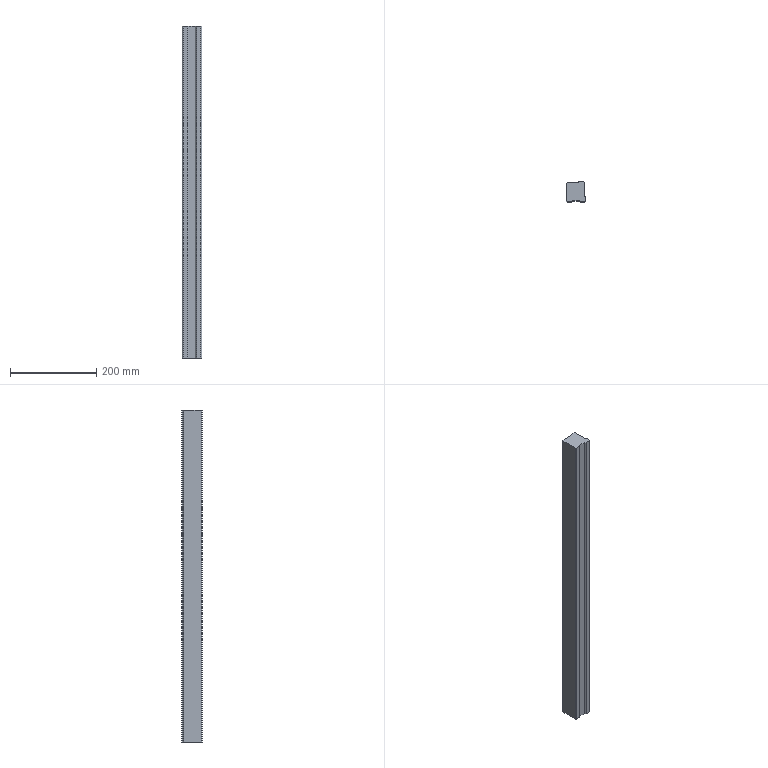Part | STEP file | Platform guide seat (default) | 1 solid | 18 faces | box 45 x 47 x 770 mm | volume 1483790 mm3 | plane 18
STEP:
#1=CARTESIAN_POINT('',(10.5,-23.5,-385.));
#2=VERTEX_POINT('',#1);
#3=CARTESIAN_POINT('',(20.5,-23.5,-385.));
#4=VERTEX_POINT('',#3);
#5=CARTESIAN_POINT('',(-22.5,-23.5,-385.));
#6=DIRECTION('',(1.,0.,0.));
#7=VECTOR('',#6,1000.);
#8=LINE('',#5,#7);
#9=EDGE_CURVE('',#2,#4,#8,.T.);
#10=ORIENTED_EDGE('',*,*,#9,.T.);
#11=CARTESIAN_POINT('',(20.5,-23.5,385.));
#12=VERTEX_POINT('',#11);
#13=CARTESIAN_POINT('',(20.5,-23.5,385.));
#14=DIRECTION('',(0.,0.,1.));
#15=VECTOR('',#14,1000.);
#16=LINE('',#13,#15);
#17=EDGE_CURVE('',#4,#12,#16,.T.);
#18=ORIENTED_EDGE('',*,*,#17,.T.);
#19=CARTESIAN_POINT('',(10.5,-23.5,385.));
#20=VERTEX_POINT('',#19);
#21=CARTESIAN_POINT('',(-22.5,-23.5,385.));
#22=DIRECTION('',(1.,0.,0.));
#23=VECTOR('',#22,1000.);
#24=LINE('',#21,#23);
#25=EDGE_CURVE('',#20,#12,#24,.T.);
#26=ORIENTED_EDGE('',*,*,#25,.F.);
#27=CARTESIAN_POINT('',(10.5,-23.5,-385.));
#28=DIRECTION('',(0.,0.,1.));
#29=VECTOR('',#28,1000.);
#30=LINE('',#27,#29);
#31=EDGE_CURVE('',#2,#20,#30,.T.);
#32=ORIENTED_EDGE('',*,*,#31,.F.);
#33=EDGE_LOOP('',(#10,#18,#26,#32));
#34=FACE_OUTER_BOUND('',#33,.T.);
#35=CARTESIAN_POINT('',(-22.5,-23.5,385.));
#36=DIRECTION('',(0.,1.,0.));
#37=DIRECTION('',(0.,0.,1.));
#38=AXIS2_PLACEMENT_3D('',#35,#36,#37);
#39=PLANE('',#38);
#40=ADVANCED_FACE('',(#34),#39,.F.);
#41=CARTESIAN_POINT('',(22.5,-21.5,385.));
#42=VERTEX_POINT('',#41);
#43=CARTESIAN_POINT('',(22.5,-11.5,385.));
#44=VERTEX_POINT('',#43);
#45=CARTESIAN_POINT('',(22.5,23.5,385.));
#46=DIRECTION('',(0.,1.,0.));
#47=VECTOR('',#46,1000.);
#48=LINE('',#45,#47);
#49=EDGE_CURVE('',#42,#44,#48,.T.);
#50=ORIENTED_EDGE('',*,*,#49,.F.);
#51=CARTESIAN_POINT('',(22.5,-21.5,-385.));
#52=VERTEX_POINT('',#51);
#53=CARTESIAN_POINT('',(22.5,-21.5,385.));
#54=DIRECTION('',(0.,0.,-1.));
#55=VECTOR('',#54,1000.);
#56=LINE('',#53,#55);
#57=EDGE_CURVE('',#42,#52,#56,.T.);
#58=ORIENTED_EDGE('',*,*,#57,.T.);
#59=CARTESIAN_POINT('',(22.5,-11.5,-385.));
#60=VERTEX_POINT('',#59);
#61=CARTESIAN_POINT('',(22.5,23.5,-385.));
#62=DIRECTION('',(0.,1.,0.));
#63=VECTOR('',#62,1000.);
#64=LINE('',#61,#63);
#65=EDGE_CURVE('',#52,#60,#64,.T.);
#66=ORIENTED_EDGE('',*,*,#65,.T.);
#67=CARTESIAN_POINT('',(22.5,-11.5,-385.));
#68=DIRECTION('',(0.,0.,1.));
#69=VECTOR('',#68,1000.);
#70=LINE('',#67,#69);
#71=EDGE_CURVE('',#60,#44,#70,.T.);
#72=ORIENTED_EDGE('',*,*,#71,.T.);
#73=EDGE_LOOP('',(#50,#58,#66,#72));
#74=FACE_OUTER_BOUND('',#73,.T.);
#75=CARTESIAN_POINT('',(22.5,23.5,385.));
#76=DIRECTION('',(-1.,0.,0.));
#77=DIRECTION('',(0.,-1.,0.));
#78=AXIS2_PLACEMENT_3D('',#75,#76,#77);
#79=PLANE('',#78);
#80=ADVANCED_FACE('',(#74),#79,.F.);
#81=CARTESIAN_POINT('',(18.5,23.5,385.));
#82=VERTEX_POINT('',#81);
#83=CARTESIAN_POINT('',(5.5,23.5,385.));
#84=VERTEX_POINT('',#83);
#85=CARTESIAN_POINT('',(-22.5,23.5,385.));
#86=DIRECTION('',(-1.,0.,0.));
#87=VECTOR('',#86,1000.);
#88=LINE('',#85,#87);
#89=EDGE_CURVE('',#82,#84,#88,.T.);
#90=ORIENTED_EDGE('',*,*,#89,.F.);
#91=CARTESIAN_POINT('',(18.5,23.5,-385.));
#92=VERTEX_POINT('',#91);
#93=CARTESIAN_POINT('',(18.5,23.5,385.));
#94=DIRECTION('',(0.,0.,-1.));
#95=VECTOR('',#94,1000.);
#96=LINE('',#93,#95);
#97=EDGE_CURVE('',#82,#92,#96,.T.);
#98=ORIENTED_EDGE('',*,*,#97,.T.);
#99=CARTESIAN_POINT('',(5.5,23.5,-385.));
#100=VERTEX_POINT('',#99);
#101=CARTESIAN_POINT('',(-22.5,23.5,-385.));
#102=DIRECTION('',(-1.,0.,0.));
#103=VECTOR('',#102,1000.);
#104=LINE('',#101,#103);
#105=EDGE_CURVE('',#92,#100,#104,.T.);
#106=ORIENTED_EDGE('',*,*,#105,.T.);
#107=CARTESIAN_POINT('',(5.5,23.5,-385.));
#108=DIRECTION('',(0.,0.,1.));
#109=VECTOR('',#108,1000.);
#110=LINE('',#107,#109);
#111=EDGE_CURVE('',#100,#84,#110,.T.);
#112=ORIENTED_EDGE('',*,*,#111,.T.);
#113=EDGE_LOOP('',(#90,#98,#106,#112));
#114=FACE_OUTER_BOUND('',#113,.T.);
#115=CARTESIAN_POINT('',(-22.5,23.5,385.));
#116=DIRECTION('',(0.,-1.,0.));
#117=DIRECTION('',(0.,0.,-1.));
#118=AXIS2_PLACEMENT_3D('',#115,#116,#117);
#119=PLANE('',#118);
#120=ADVANCED_FACE('',(#114),#119,.F.);
#121=CARTESIAN_POINT('',(-22.5,19.5,385.));
#122=VERTEX_POINT('',#121);
#123=CARTESIAN_POINT('',(-22.5,-21.5,385.));
#124=VERTEX_POINT('',#123);
#125=CARTESIAN_POINT('',(-22.5,23.5,385.));
#126=DIRECTION('',(0.,-1.,0.));
#127=VECTOR('',#126,1000.);
#128=LINE('',#125,#127);
#129=EDGE_CURVE('',#122,#124,#128,.T.);
#130=ORIENTED_EDGE('',*,*,#129,.F.);
#131=CARTESIAN_POINT('',(-22.5,19.5,-385.));
#132=VERTEX_POINT('',#131);
#133=CARTESIAN_POINT('',(-22.5,19.5,385.));
#134=DIRECTION('',(0.,0.,-1.));
#135=VECTOR('',#134,1000.);
#136=LINE('',#133,#135);
#137=EDGE_CURVE('',#122,#132,#136,.T.);
#138=ORIENTED_EDGE('',*,*,#137,.T.);
#139=CARTESIAN_POINT('',(-22.5,-21.5,-385.));
#140=VERTEX_POINT('',#139);
#141=CARTESIAN_POINT('',(-22.5,23.5,-385.));
#142=DIRECTION('',(0.,-1.,0.));
#143=VECTOR('',#142,1000.);
#144=LINE('',#141,#143);
#145=EDGE_CURVE('',#132,#140,#144,.T.);
#146=ORIENTED_EDGE('',*,*,#145,.T.);
#147=CARTESIAN_POINT('',(-22.5,-21.5,385.));
#148=DIRECTION('',(0.,0.,1.));
#149=VECTOR('',#148,1000.);
#150=LINE('',#147,#149);
#151=EDGE_CURVE('',#140,#124,#150,.T.);
#152=ORIENTED_EDGE('',*,*,#151,.T.);
#153=EDGE_LOOP('',(#130,#138,#146,#152));
#154=FACE_OUTER_BOUND('',#153,.T.);
#155=CARTESIAN_POINT('',(-22.5,23.5,385.));
#156=DIRECTION('',(1.,0.,0.));
#157=DIRECTION('',(0.,1.,0.));
#158=AXIS2_PLACEMENT_3D('',#155,#156,#157);
#159=PLANE('',#158);
#160=ADVANCED_FACE('',(#154),#159,.F.);
#161=CARTESIAN_POINT('',(-20.5,-23.5,385.));
#162=VERTEX_POINT('',#161);
#163=CARTESIAN_POINT('',(-10.5,-23.5,385.));
#164=VERTEX_POINT('',#163);
#165=CARTESIAN_POINT('',(-22.5,-23.5,385.));
#166=DIRECTION('',(1.,0.,0.));
#167=VECTOR('',#166,1000.);
#168=LINE('',#165,#167);
#169=EDGE_CURVE('',#162,#164,#168,.T.);
#170=ORIENTED_EDGE('',*,*,#169,.F.);
#171=CARTESIAN_POINT('',(-20.5,-23.5,-385.));
#172=VERTEX_POINT('',#171);
#173=CARTESIAN_POINT('',(-20.5,-23.5,385.));
#174=DIRECTION('',(0.,0.,-1.));
#175=VECTOR('',#174,1000.);
#176=LINE('',#173,#175);
#177=EDGE_CURVE('',#162,#172,#176,.T.);
#178=ORIENTED_EDGE('',*,*,#177,.T.);
#179=CARTESIAN_POINT('',(-10.5,-23.5,-385.));
#180=VERTEX_POINT('',#179);
#181=CARTESIAN_POINT('',(-22.5,-23.5,-385.));
#182=DIRECTION('',(1.,0.,0.));
#183=VECTOR('',#182,1000.);
#184=LINE('',#181,#183);
#185=EDGE_CURVE('',#172,#180,#184,.T.);
#186=ORIENTED_EDGE('',*,*,#185,.T.);
#187=CARTESIAN_POINT('',(-10.5,-23.5,-385.));
#188=DIRECTION('',(0.,0.,1.));
#189=VECTOR('',#188,1000.);
#190=LINE('',#187,#189);
#191=EDGE_CURVE('',#180,#164,#190,.T.);
#192=ORIENTED_EDGE('',*,*,#191,.T.);
#193=EDGE_LOOP('',(#170,#178,#186,#192));
#194=FACE_OUTER_BOUND('',#193,.T.);
#195=CARTESIAN_POINT('',(-22.5,-23.5,385.));
#196=DIRECTION('',(0.,1.,0.));
#197=DIRECTION('',(0.,0.,1.));
#198=AXIS2_PLACEMENT_3D('',#195,#196,#197);
#199=PLANE('',#198);
#200=ADVANCED_FACE('',(#194),#199,.F.);
#201=CARTESIAN_POINT('',(20.5,21.5,385.));
#202=VERTEX_POINT('',#201);
#203=CARTESIAN_POINT('',(20.5,-11.5,385.));
#204=VERTEX_POINT('',#203);
#205=CARTESIAN_POINT('',(20.5,23.5,385.));
#206=DIRECTION('',(0.,-1.,0.));
#207=VECTOR('',#206,1000.);
#208=LINE('',#205,#207);
#209=EDGE_CURVE('',#202,#204,#208,.T.);
#210=ORIENTED_EDGE('',*,*,#209,.F.);
#211=CARTESIAN_POINT('',(21.,21.,385.));
#212=DIRECTION('',(-0.7071,0.7071,0.));
#213=VECTOR('',#212,1000.);
#214=LINE('',#211,#213);
#215=EDGE_CURVE('',#202,#82,#214,.T.);
#216=ORIENTED_EDGE('',*,*,#215,.T.);
#217=ORIENTED_EDGE('',*,*,#89,.T.);
#218=CARTESIAN_POINT('',(5.5,21.5,385.));
#219=VERTEX_POINT('',#218);
#220=CARTESIAN_POINT('',(5.5,23.5,385.));
#221=DIRECTION('',(0.,1.,0.));
#222=VECTOR('',#221,1000.);
#223=LINE('',#220,#222);
#224=EDGE_CURVE('',#219,#84,#223,.T.);
#225=ORIENTED_EDGE('',*,*,#224,.F.);
#226=CARTESIAN_POINT('',(-20.5,21.5,385.));
#227=VERTEX_POINT('',#226);
#228=CARTESIAN_POINT('',(-22.5,21.5,385.));
#229=DIRECTION('',(1.,0.,0.));
#230=VECTOR('',#229,1000.);
#231=LINE('',#228,#230);
#232=EDGE_CURVE('',#227,#219,#231,.T.);
#233=ORIENTED_EDGE('',*,*,#232,.F.);
#234=CARTESIAN_POINT('',(-21.,21.,385.));
#235=DIRECTION('',(-0.7071,-0.7071,0.));
#236=VECTOR('',#235,1000.);
#237=LINE('',#234,#236);
#238=EDGE_CURVE('',#227,#122,#237,.T.);
#239=ORIENTED_EDGE('',*,*,#238,.T.);
#240=ORIENTED_EDGE('',*,*,#129,.T.);
#241=CARTESIAN_POINT('',(-22.,-22.,385.));
#242=DIRECTION('',(0.7071,-0.7071,0.));
#243=VECTOR('',#242,1000.);
#244=LINE('',#241,#243);
#245=EDGE_CURVE('',#124,#162,#244,.T.);
#246=ORIENTED_EDGE('',*,*,#245,.T.);
#247=ORIENTED_EDGE('',*,*,#169,.T.);
#248=CARTESIAN_POINT('',(-7.5,-20.5,385.));
#249=VERTEX_POINT('',#248);
#250=CARTESIAN_POINT('',(-7.5,-20.5,385.));
#251=DIRECTION('',(-0.7071,-0.7071,0.));
#252=VECTOR('',#251,1000.);
#253=LINE('',#250,#252);
#254=EDGE_CURVE('',#249,#164,#253,.T.);
#255=ORIENTED_EDGE('',*,*,#254,.F.);
#256=CARTESIAN_POINT('',(7.5,-20.5,385.));
#257=VERTEX_POINT('',#256);
#258=CARTESIAN_POINT('',(-7.5,-20.5,385.));
#259=DIRECTION('',(-1.,0.,0.));
#260=VECTOR('',#259,1000.);
#261=LINE('',#258,#260);
#262=EDGE_CURVE('',#257,#249,#261,.T.);
#263=ORIENTED_EDGE('',*,*,#262,.F.);
#264=CARTESIAN_POINT('',(7.5,-20.5,385.));
#265=DIRECTION('',(-0.7071,0.7071,0.));
#266=VECTOR('',#265,1000.);
#267=LINE('',#264,#266);
#268=EDGE_CURVE('',#20,#257,#267,.T.);
#269=ORIENTED_EDGE('',*,*,#268,.F.);
#270=ORIENTED_EDGE('',*,*,#25,.T.);
#271=CARTESIAN_POINT('',(22.,-22.,385.));
#272=DIRECTION('',(0.7071,0.7071,0.));
#273=VECTOR('',#272,1000.);
#274=LINE('',#271,#273);
#275=EDGE_CURVE('',#12,#42,#274,.T.);
#276=ORIENTED_EDGE('',*,*,#275,.T.);
#277=ORIENTED_EDGE('',*,*,#49,.T.);
#278=CARTESIAN_POINT('',(22.5,-11.5,385.));
#279=DIRECTION('',(1.,0.,0.));
#280=VECTOR('',#279,1000.);
#281=LINE('',#278,#280);
#282=EDGE_CURVE('',#204,#44,#281,.T.);
#283=ORIENTED_EDGE('',*,*,#282,.F.);
#284=EDGE_LOOP('',(#210,#216,#217,#225,#233,#239,#240,#246,#247,#255,#263,#269,#270,#276,#277,#283));
#285=FACE_OUTER_BOUND('',#284,.T.);
#286=CARTESIAN_POINT('',(0.,0.,385.));
#287=DIRECTION('',(0.,0.,1.));
#288=DIRECTION('',(1.,0.,0.));
#289=AXIS2_PLACEMENT_3D('',#286,#287,#288);
#290=PLANE('',#289);
#291=ADVANCED_FACE('',(#285),#290,.T.);
#292=ORIENTED_EDGE('',*,*,#105,.F.);
#293=CARTESIAN_POINT('',(20.5,21.5,-385.));
#294=VERTEX_POINT('',#293);
#295=CARTESIAN_POINT('',(20.5,21.5,-385.));
#296=DIRECTION('',(0.7071,-0.7071,0.));
#297=VECTOR('',#296,1000.);
#298=LINE('',#295,#297);
#299=EDGE_CURVE('',#92,#294,#298,.T.);
#300=ORIENTED_EDGE('',*,*,#299,.T.);
#301=CARTESIAN_POINT('',(20.5,-11.5,-385.));
#302=VERTEX_POINT('',#301);
#303=CARTESIAN_POINT('',(20.5,23.5,-385.));
#304=DIRECTION('',(0.,-1.,0.));
#305=VECTOR('',#304,1000.);
#306=LINE('',#303,#305);
#307=EDGE_CURVE('',#294,#302,#306,.T.);
#308=ORIENTED_EDGE('',*,*,#307,.T.);
#309=CARTESIAN_POINT('',(22.5,-11.5,-385.));
#310=DIRECTION('',(1.,0.,0.));
#311=VECTOR('',#310,1000.);
#312=LINE('',#309,#311);
#313=EDGE_CURVE('',#302,#60,#312,.T.);
#314=ORIENTED_EDGE('',*,*,#313,.T.);
#315=ORIENTED_EDGE('',*,*,#65,.F.);
#316=CARTESIAN_POINT('',(22.5,-21.5,-385.));
#317=DIRECTION('',(-0.7071,-0.7071,0.));
#318=VECTOR('',#317,1000.);
#319=LINE('',#316,#318);
#320=EDGE_CURVE('',#52,#4,#319,.T.);
#321=ORIENTED_EDGE('',*,*,#320,.T.);
#322=ORIENTED_EDGE('',*,*,#9,.F.);
#323=CARTESIAN_POINT('',(7.5,-20.5,-385.));
#324=VERTEX_POINT('',#323);
#325=CARTESIAN_POINT('',(7.5,-20.5,-385.));
#326=DIRECTION('',(-0.7071,0.7071,0.));
#327=VECTOR('',#326,1000.);
#328=LINE('',#325,#327);
#329=EDGE_CURVE('',#2,#324,#328,.T.);
#330=ORIENTED_EDGE('',*,*,#329,.T.);
#331=CARTESIAN_POINT('',(-7.5,-20.5,-385.));
#332=VERTEX_POINT('',#331);
#333=CARTESIAN_POINT('',(-7.5,-20.5,-385.));
#334=DIRECTION('',(-1.,0.,0.));
#335=VECTOR('',#334,1000.);
#336=LINE('',#333,#335);
#337=EDGE_CURVE('',#324,#332,#336,.T.);
#338=ORIENTED_EDGE('',*,*,#337,.T.);
#339=CARTESIAN_POINT('',(-7.5,-20.5,-385.));
#340=DIRECTION('',(-0.7071,-0.7071,0.));
#341=VECTOR('',#340,1000.);
#342=LINE('',#339,#341);
#343=EDGE_CURVE('',#332,#180,#342,.T.);
#344=ORIENTED_EDGE('',*,*,#343,.T.);
#345=ORIENTED_EDGE('',*,*,#185,.F.);
#346=CARTESIAN_POINT('',(-20.5,-23.5,-385.));
#347=DIRECTION('',(-0.7071,0.7071,0.));
#348=VECTOR('',#347,1000.);
#349=LINE('',#346,#348);
#350=EDGE_CURVE('',#172,#140,#349,.T.);
#351=ORIENTED_EDGE('',*,*,#350,.T.);
#352=ORIENTED_EDGE('',*,*,#145,.F.);
#353=CARTESIAN_POINT('',(-20.5,21.5,-385.));
#354=VERTEX_POINT('',#353);
#355=CARTESIAN_POINT('',(-20.5,21.5,-385.));
#356=DIRECTION('',(0.7071,0.7071,0.));
#357=VECTOR('',#356,1000.);
#358=LINE('',#355,#357);
#359=EDGE_CURVE('',#132,#354,#358,.T.);
#360=ORIENTED_EDGE('',*,*,#359,.T.);
#361=CARTESIAN_POINT('',(5.5,21.5,-385.));
#362=VERTEX_POINT('',#361);
#363=CARTESIAN_POINT('',(-22.5,21.5,-385.));
#364=DIRECTION('',(1.,0.,0.));
#365=VECTOR('',#364,1000.);
#366=LINE('',#363,#365);
#367=EDGE_CURVE('',#354,#362,#366,.T.);
#368=ORIENTED_EDGE('',*,*,#367,.T.);
#369=CARTESIAN_POINT('',(5.5,23.5,-385.));
#370=DIRECTION('',(0.,1.,0.));
#371=VECTOR('',#370,1000.);
#372=LINE('',#369,#371);
#373=EDGE_CURVE('',#362,#100,#372,.T.);
#374=ORIENTED_EDGE('',*,*,#373,.T.);
#375=EDGE_LOOP('',(#292,#300,#308,#314,#315,#321,#322,#330,#338,#344,#345,#351,#352,#360,#368,#374));
#376=FACE_OUTER_BOUND('',#375,.T.);
#377=CARTESIAN_POINT('',(0.,0.,-385.));
#378=DIRECTION('',(0.,0.,1.));
#379=DIRECTION('',(1.,0.,0.));
#380=AXIS2_PLACEMENT_3D('',#377,#378,#379);
#381=PLANE('',#380);
#382=ADVANCED_FACE('',(#376),#381,.F.);
#383=ORIENTED_EDGE('',*,*,#224,.T.);
#384=ORIENTED_EDGE('',*,*,#111,.F.);
#385=ORIENTED_EDGE('',*,*,#373,.F.);
#386=CARTESIAN_POINT('',(5.5,21.5,-385.));
#387=DIRECTION('',(0.,0.,1.));
#388=VECTOR('',#387,1000.);
#389=LINE('',#386,#388);
#390=EDGE_CURVE('',#362,#219,#389,.T.);
#391=ORIENTED_EDGE('',*,*,#390,.T.);
#392=EDGE_LOOP('',(#383,#384,#385,#391));
#393=FACE_OUTER_BOUND('',#392,.T.);
#394=CARTESIAN_POINT('',(5.5,23.5,-385.));
#395=DIRECTION('',(1.,0.,0.));
#396=DIRECTION('',(0.,0.,-1.));
#397=AXIS2_PLACEMENT_3D('',#394,#395,#396);
#398=PLANE('',#397);
#399=ADVANCED_FACE('',(#393),#398,.F.);
#400=ORIENTED_EDGE('',*,*,#367,.F.);
#401=CARTESIAN_POINT('',(-20.5,21.5,-385.));
#402=DIRECTION('',(0.,0.,1.));
#403=VECTOR('',#402,1000.);
#404=LINE('',#401,#403);
#405=EDGE_CURVE('',#354,#227,#404,.T.);
#406=ORIENTED_EDGE('',*,*,#405,.T.);
#407=ORIENTED_EDGE('',*,*,#232,.T.);
#408=ORIENTED_EDGE('',*,*,#390,.F.);
#409=EDGE_LOOP('',(#400,#406,#407,#408));
#410=FACE_OUTER_BOUND('',#409,.T.);
#411=CARTESIAN_POINT('',(-22.5,21.5,-385.));
#412=DIRECTION('',(0.,-1.,0.));
#413=DIRECTION('',(0.,0.,-1.));
#414=AXIS2_PLACEMENT_3D('',#411,#412,#413);
#415=PLANE('',#414);
#416=ADVANCED_FACE('',(#410),#415,.F.);
#417=ORIENTED_EDGE('',*,*,#282,.T.);
#418=ORIENTED_EDGE('',*,*,#71,.F.);
#419=ORIENTED_EDGE('',*,*,#313,.F.);
#420=CARTESIAN_POINT('',(20.5,-11.5,-385.));
#421=DIRECTION('',(0.,0.,1.));
#422=VECTOR('',#421,1000.);
#423=LINE('',#420,#422);
#424=EDGE_CURVE('',#302,#204,#423,.T.);
#425=ORIENTED_EDGE('',*,*,#424,.T.);
#426=EDGE_LOOP('',(#417,#418,#419,#425));
#427=FACE_OUTER_BOUND('',#426,.T.);
#428=CARTESIAN_POINT('',(22.5,-11.5,-385.));
#429=DIRECTION('',(0.,-1.,0.));
#430=DIRECTION('',(0.,0.,-1.));
#431=AXIS2_PLACEMENT_3D('',#428,#429,#430);
#432=PLANE('',#431);
#433=ADVANCED_FACE('',(#427),#432,.F.);
#434=ORIENTED_EDGE('',*,*,#307,.F.);
#435=CARTESIAN_POINT('',(20.5,21.5,-385.));
#436=DIRECTION('',(0.,0.,1.));
#437=VECTOR('',#436,1000.);
#438=LINE('',#435,#437);
#439=EDGE_CURVE('',#294,#202,#438,.T.);
#440=ORIENTED_EDGE('',*,*,#439,.T.);
#441=ORIENTED_EDGE('',*,*,#209,.T.);
#442=ORIENTED_EDGE('',*,*,#424,.F.);
#443=EDGE_LOOP('',(#434,#440,#441,#442));
#444=FACE_OUTER_BOUND('',#443,.T.);
#445=CARTESIAN_POINT('',(20.5,23.5,-385.));
#446=DIRECTION('',(-1.,0.,0.));
#447=DIRECTION('',(0.,-1.,0.));
#448=AXIS2_PLACEMENT_3D('',#445,#446,#447);
#449=PLANE('',#448);
#450=ADVANCED_FACE('',(#444),#449,.F.);
#451=ORIENTED_EDGE('',*,*,#268,.T.);
#452=CARTESIAN_POINT('',(7.5,-20.5,-385.));
#453=DIRECTION('',(0.,0.,1.));
#454=VECTOR('',#453,1000.);
#455=LINE('',#452,#454);
#456=EDGE_CURVE('',#324,#257,#455,.T.);
#457=ORIENTED_EDGE('',*,*,#456,.F.);
#458=ORIENTED_EDGE('',*,*,#329,.F.);
#459=ORIENTED_EDGE('',*,*,#31,.T.);
#460=EDGE_LOOP('',(#451,#457,#458,#459));
#461=FACE_OUTER_BOUND('',#460,.T.);
#462=CARTESIAN_POINT('',(7.5,-20.5,-385.));
#463=DIRECTION('',(0.7071,0.7071,0.));
#464=DIRECTION('',(-0.7071,0.7071,0.));
#465=AXIS2_PLACEMENT_3D('',#462,#463,#464);
#466=PLANE('',#465);
#467=ADVANCED_FACE('',(#461),#466,.F.);
#468=ORIENTED_EDGE('',*,*,#254,.T.);
#469=ORIENTED_EDGE('',*,*,#191,.F.);
#470=ORIENTED_EDGE('',*,*,#343,.F.);
#471=CARTESIAN_POINT('',(-7.5,-20.5,-385.));
#472=DIRECTION('',(0.,0.,1.));
#473=VECTOR('',#472,1000.);
#474=LINE('',#471,#473);
#475=EDGE_CURVE('',#332,#249,#474,.T.);
#476=ORIENTED_EDGE('',*,*,#475,.T.);
#477=EDGE_LOOP('',(#468,#469,#470,#476));
#478=FACE_OUTER_BOUND('',#477,.T.);
#479=CARTESIAN_POINT('',(-7.5,-20.5,-385.));
#480=DIRECTION('',(-0.7071,0.7071,0.));
#481=DIRECTION('',(-0.7071,-0.7071,0.));
#482=AXIS2_PLACEMENT_3D('',#479,#480,#481);
#483=PLANE('',#482);
#484=ADVANCED_FACE('',(#478),#483,.F.);
#485=ORIENTED_EDGE('',*,*,#262,.T.);
#486=ORIENTED_EDGE('',*,*,#475,.F.);
#487=ORIENTED_EDGE('',*,*,#337,.F.);
#488=ORIENTED_EDGE('',*,*,#456,.T.);
#489=EDGE_LOOP('',(#485,#486,#487,#488));
#490=FACE_OUTER_BOUND('',#489,.T.);
#491=CARTESIAN_POINT('',(-7.5,-20.5,-385.));
#492=DIRECTION('',(0.,1.,0.));
#493=DIRECTION('',(0.,0.,1.));
#494=AXIS2_PLACEMENT_3D('',#491,#492,#493);
#495=PLANE('',#494);
#496=ADVANCED_FACE('',(#490),#495,.F.);
#497=ORIENTED_EDGE('',*,*,#299,.F.);
#498=ORIENTED_EDGE('',*,*,#97,.F.);
#499=ORIENTED_EDGE('',*,*,#215,.F.);
#500=ORIENTED_EDGE('',*,*,#439,.F.);
#501=EDGE_LOOP('',(#497,#498,#499,#500));
#502=FACE_OUTER_BOUND('',#501,.T.);
#503=CARTESIAN_POINT('',(20.5,21.5,-385.));
#504=DIRECTION('',(-0.7071,-0.7071,0.));
#505=DIRECTION('',(0.,0.,1.));
#506=AXIS2_PLACEMENT_3D('',#503,#504,#505);
#507=PLANE('',#506);
#508=ADVANCED_FACE('',(#502),#507,.F.);
#509=ORIENTED_EDGE('',*,*,#359,.F.);
#510=ORIENTED_EDGE('',*,*,#137,.F.);
#511=ORIENTED_EDGE('',*,*,#238,.F.);
#512=ORIENTED_EDGE('',*,*,#405,.F.);
#513=EDGE_LOOP('',(#509,#510,#511,#512));
#514=FACE_OUTER_BOUND('',#513,.T.);
#515=CARTESIAN_POINT('',(-20.5,21.5,-385.));
#516=DIRECTION('',(0.7071,-0.7071,0.));
#517=DIRECTION('',(0.,0.,1.));
#518=AXIS2_PLACEMENT_3D('',#515,#516,#517);
#519=PLANE('',#518);
#520=ADVANCED_FACE('',(#514),#519,.F.);
#521=ORIENTED_EDGE('',*,*,#245,.F.);
#522=ORIENTED_EDGE('',*,*,#151,.F.);
#523=ORIENTED_EDGE('',*,*,#350,.F.);
#524=ORIENTED_EDGE('',*,*,#177,.F.);
#525=EDGE_LOOP('',(#521,#522,#523,#524));
#526=FACE_OUTER_BOUND('',#525,.T.);
#527=CARTESIAN_POINT('',(-20.5,-23.5,385.));
#528=DIRECTION('',(0.7071,0.7071,0.));
#529=DIRECTION('',(0.,0.,-1.));
#530=AXIS2_PLACEMENT_3D('',#527,#528,#529);
#531=PLANE('',#530);
#532=ADVANCED_FACE('',(#526),#531,.F.);
#533=ORIENTED_EDGE('',*,*,#275,.F.);
#534=ORIENTED_EDGE('',*,*,#17,.F.);
#535=ORIENTED_EDGE('',*,*,#320,.F.);
#536=ORIENTED_EDGE('',*,*,#57,.F.);
#537=EDGE_LOOP('',(#533,#534,#535,#536));
#538=FACE_OUTER_BOUND('',#537,.T.);
#539=CARTESIAN_POINT('',(22.5,-21.5,385.));
#540=DIRECTION('',(-0.7071,0.7071,0.));
#541=DIRECTION('',(0.,0.,-1.));
#542=AXIS2_PLACEMENT_3D('',#539,#540,#541);
#543=PLANE('',#542);
#544=ADVANCED_FACE('',(#538),#543,.F.);
#545=CLOSED_SHELL('',(#40,#80,#120,#160,#200,#291,#382,#399,#416,#433,#450,#467,#484,#496,#508,#520,#532,#544));
#546=MANIFOLD_SOLID_BREP('',#545);
#547=CARTESIAN_POINT('',(0.,0.,0.));
#548=DIRECTION('',(0.,0.,1.));
#549=DIRECTION('',(1.,0.,0.));
#550=AXIS2_PLACEMENT_3D('',#547,#548,#549);
#551=(LENGTH_UNIT()NAMED_UNIT(*)SI_UNIT(.MILLI.,.METRE.));
#552=UNCERTAINTY_MEASURE_WITH_UNIT(LENGTH_MEASURE(0.00001),#551,'','');
#553=(NAMED_UNIT(*)PLANE_ANGLE_UNIT()SI_UNIT($,.RADIAN.));
#554=(NAMED_UNIT(*)SI_UNIT($,.STERADIAN.)SOLID_ANGLE_UNIT());
#555=(GEOMETRIC_REPRESENTATION_CONTEXT(3)GLOBAL_UNCERTAINTY_ASSIGNED_CONTEXT((#552))GLOBAL_UNIT_ASSIGNED_CONTEXT((#551,#553,#554))REPRESENTATION_CONTEXT('',''));
#556=ADVANCED_BREP_SHAPE_REPRESENTATION('',(#546,#550),#555);